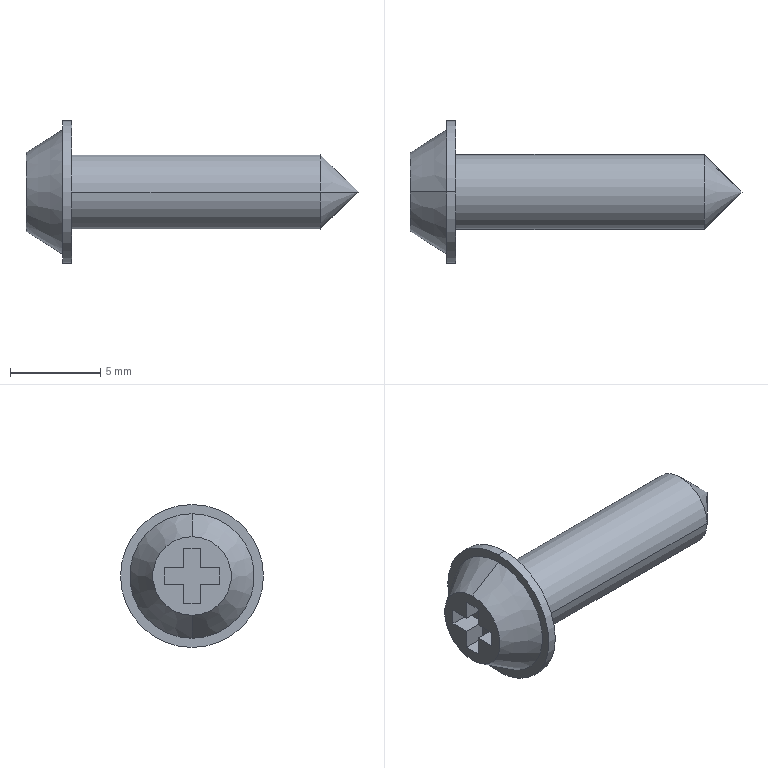Part | NX | features BREP 1 | 1 solid | 24 faces | box 18.415 x 7.925 x 7.925 mm | volume 268.123 mm3 | plane 16 | cylinder 4 | cone 4 | commonest cylinder face diameters 4.166 x2 7.925 x2
STEP:
#1=CARTESIAN_POINT('',(-15.875,2.083,0.));
#2=VERTEX_POINT('',#1);
#3=CARTESIAN_POINT('',(-2.083,2.083,0.));
#4=VERTEX_POINT('',#3);
#5=CARTESIAN_POINT('',(-2.083,2.083,0.));
#6=DIRECTION('',(-1.,0.,0.));
#7=VECTOR('',#6,1000.);
#8=LINE('',#5,#7);
#9=EDGE_CURVE('',#2,#4,#8,.F.);
#10=ORIENTED_EDGE('',*,*,#9,.T.);
#11=CARTESIAN_POINT('',(-2.083,-2.083,0.));
#12=VERTEX_POINT('',#11);
#13=CARTESIAN_POINT('',(-2.083,0.,0.));
#14=DIRECTION('',(-1.,0.,0.));
#15=DIRECTION('',(0.,1.,0.));
#16=AXIS2_PLACEMENT_3D('',#13,#14,#15);
#17=CIRCLE('',#16,2.083);
#18=EDGE_CURVE('',#4,#12,#17,.T.);
#19=ORIENTED_EDGE('',*,*,#18,.T.);
#20=CARTESIAN_POINT('',(-15.875,-2.083,0.));
#21=VERTEX_POINT('',#20);
#22=CARTESIAN_POINT('',(-2.083,-2.083,0.));
#23=DIRECTION('',(-1.,0.,0.));
#24=VECTOR('',#23,1000.);
#25=LINE('',#22,#24);
#26=EDGE_CURVE('',#21,#12,#25,.F.);
#27=ORIENTED_EDGE('',*,*,#26,.F.);
#28=CARTESIAN_POINT('',(-15.875,0.,0.));
#29=DIRECTION('',(-1.,0.,0.));
#30=DIRECTION('',(0.,1.,0.));
#31=AXIS2_PLACEMENT_3D('',#28,#29,#30);
#32=CIRCLE('',#31,2.083);
#33=EDGE_CURVE('',#2,#21,#32,.T.);
#34=ORIENTED_EDGE('',*,*,#33,.F.);
#35=EDGE_LOOP('',(#10,#19,#27,#34));
#36=FACE_BOUND('',#35,.T.);
#37=CARTESIAN_POINT('',(0.,0.,0.));
#38=DIRECTION('',(-1.,0.,0.));
#39=DIRECTION('',(0.,1.,0.));
#40=AXIS2_PLACEMENT_3D('',#37,#38,#39);
#41=CYLINDRICAL_SURFACE('',#40,2.083);
#42=ADVANCED_FACE('',(#36),#41,.T.);
#43=CARTESIAN_POINT('',(-15.875,0.,-3.962));
#44=VERTEX_POINT('',#43);
#45=CARTESIAN_POINT('',(-15.875,0.,3.962));
#46=VERTEX_POINT('',#45);
#47=CARTESIAN_POINT('',(-15.875,0.,0.));
#48=DIRECTION('',(-1.,0.,0.));
#49=DIRECTION('',(0.,0.,-1.));
#50=AXIS2_PLACEMENT_3D('',#47,#48,#49);
#51=CIRCLE('',#50,3.962);
#52=EDGE_CURVE('',#44,#46,#51,.T.);
#53=ORIENTED_EDGE('',*,*,#52,.F.);
#54=CARTESIAN_POINT('',(-15.875,0.,0.));
#55=DIRECTION('',(1.,0.,0.));
#56=DIRECTION('',(0.,0.,-1.));
#57=AXIS2_PLACEMENT_3D('',#54,#55,#56);
#58=CIRCLE('',#57,3.962);
#59=EDGE_CURVE('',#44,#46,#58,.T.);
#60=ORIENTED_EDGE('',*,*,#59,.T.);
#61=EDGE_LOOP('',(#53,#60));
#62=FACE_BOUND('',#61,.T.);
#63=CARTESIAN_POINT('',(-15.875,0.,0.));
#64=DIRECTION('',(-1.,0.,0.));
#65=DIRECTION('',(0.,-1.,0.));
#66=AXIS2_PLACEMENT_3D('',#63,#64,#65);
#67=CIRCLE('',#66,2.083);
#68=EDGE_CURVE('',#21,#2,#67,.T.);
#69=ORIENTED_EDGE('',*,*,#68,.T.);
#70=ORIENTED_EDGE('',*,*,#33,.T.);
#71=EDGE_LOOP('',(#69,#70));
#72=FACE_BOUND('',#71,.T.);
#73=CARTESIAN_POINT('',(-15.875,0.,0.));
#74=DIRECTION('',(-1.,0.,0.));
#75=DIRECTION('',(0.,0.,1.));
#76=AXIS2_PLACEMENT_3D('',#73,#74,#75);
#77=PLANE('',#76);
#78=ADVANCED_FACE('',(#62,#72),#77,.F.);
#79=CARTESIAN_POINT('',(-16.383,0.,-3.962));
#80=VERTEX_POINT('',#79);
#81=CARTESIAN_POINT('',(-16.383,0.,3.962));
#82=VERTEX_POINT('',#81);
#83=CARTESIAN_POINT('',(-16.383,0.,0.));
#84=DIRECTION('',(1.,0.,0.));
#85=DIRECTION('',(0.,0.,-1.));
#86=AXIS2_PLACEMENT_3D('',#83,#84,#85);
#87=CIRCLE('',#86,3.962);
#88=EDGE_CURVE('',#80,#82,#87,.T.);
#89=ORIENTED_EDGE('',*,*,#88,.T.);
#90=CARTESIAN_POINT('',(-16.383,0.,3.962));
#91=DIRECTION('',(1.,0.,0.));
#92=VECTOR('',#91,1000.);
#93=LINE('',#90,#92);
#94=EDGE_CURVE('',#82,#46,#93,.T.);
#95=ORIENTED_EDGE('',*,*,#94,.T.);
#96=ORIENTED_EDGE('',*,*,#59,.F.);
#97=CARTESIAN_POINT('',(-16.383,0.,-3.962));
#98=DIRECTION('',(1.,0.,0.));
#99=VECTOR('',#98,1000.);
#100=LINE('',#97,#99);
#101=EDGE_CURVE('',#80,#44,#100,.T.);
#102=ORIENTED_EDGE('',*,*,#101,.F.);
#103=EDGE_LOOP('',(#89,#95,#96,#102));
#104=FACE_BOUND('',#103,.T.);
#105=CARTESIAN_POINT('',(-15.748,0.,0.));
#106=DIRECTION('',(-1.,0.,0.));
#107=DIRECTION('',(0.,0.,1.));
#108=AXIS2_PLACEMENT_3D('',#105,#106,#107);
#109=CYLINDRICAL_SURFACE('',#108,3.962);
#110=ADVANCED_FACE('',(#104),#109,.T.);
#111=ORIENTED_EDGE('',*,*,#52,.T.);
#112=ORIENTED_EDGE('',*,*,#94,.F.);
#113=CARTESIAN_POINT('',(-16.383,0.,0.));
#114=DIRECTION('',(-1.,0.,0.));
#115=DIRECTION('',(0.,0.,-1.));
#116=AXIS2_PLACEMENT_3D('',#113,#114,#115);
#117=CIRCLE('',#116,3.962);
#118=EDGE_CURVE('',#80,#82,#117,.T.);
#119=ORIENTED_EDGE('',*,*,#118,.F.);
#120=ORIENTED_EDGE('',*,*,#101,.T.);
#121=EDGE_LOOP('',(#111,#112,#119,#120));
#122=FACE_BOUND('',#121,.T.);
#123=CARTESIAN_POINT('',(-15.748,0.,0.));
#124=DIRECTION('',(-1.,0.,0.));
#125=DIRECTION('',(0.,0.,1.));
#126=AXIS2_PLACEMENT_3D('',#123,#124,#125);
#127=CYLINDRICAL_SURFACE('',#126,3.962);
#128=ADVANCED_FACE('',(#122),#127,.T.);
#129=ORIENTED_EDGE('',*,*,#88,.F.);
#130=ORIENTED_EDGE('',*,*,#118,.T.);
#131=EDGE_LOOP('',(#129,#130));
#132=FACE_BOUND('',#131,.T.);
#133=CARTESIAN_POINT('',(-16.383,0.,-3.454));
#134=VERTEX_POINT('',#133);
#135=CARTESIAN_POINT('',(-16.383,0.,3.454));
#136=VERTEX_POINT('',#135);
#137=CARTESIAN_POINT('',(-16.383,0.,0.));
#138=DIRECTION('',(-1.,0.,0.));
#139=DIRECTION('',(0.,0.,-1.));
#140=AXIS2_PLACEMENT_3D('',#137,#138,#139);
#141=CIRCLE('',#140,3.454);
#142=EDGE_CURVE('',#134,#136,#141,.T.);
#143=ORIENTED_EDGE('',*,*,#142,.F.);
#144=CARTESIAN_POINT('',(-16.383,0.,0.));
#145=DIRECTION('',(1.,0.,0.));
#146=DIRECTION('',(0.,0.,-1.));
#147=AXIS2_PLACEMENT_3D('',#144,#145,#146);
#148=CIRCLE('',#147,3.454);
#149=EDGE_CURVE('',#134,#136,#148,.T.);
#150=ORIENTED_EDGE('',*,*,#149,.T.);
#151=EDGE_LOOP('',(#143,#150));
#152=FACE_BOUND('',#151,.T.);
#153=CARTESIAN_POINT('',(-16.383,0.,0.));
#154=DIRECTION('',(-1.,0.,0.));
#155=DIRECTION('',(0.,0.,1.));
#156=AXIS2_PLACEMENT_3D('',#153,#154,#155);
#157=PLANE('',#156);
#158=ADVANCED_FACE('',(#132,#152),#157,.T.);
#159=CARTESIAN_POINT('',(-18.415,0.,-2.179));
#160=VERTEX_POINT('',#159);
#161=CARTESIAN_POINT('',(-18.415,0.,2.179));
#162=VERTEX_POINT('',#161);
#163=CARTESIAN_POINT('',(-18.415,0.,0.));
#164=DIRECTION('',(1.,0.,0.));
#165=DIRECTION('',(0.,0.,-1.));
#166=AXIS2_PLACEMENT_3D('',#163,#164,#165);
#167=CIRCLE('',#166,2.179);
#168=EDGE_CURVE('',#160,#162,#167,.T.);
#169=ORIENTED_EDGE('',*,*,#168,.T.);
#170=CARTESIAN_POINT('',(-18.415,0.,2.179));
#171=DIRECTION('',(0.847,0.,0.5315));
#172=VECTOR('',#171,1000.);
#173=LINE('',#170,#172);
#174=EDGE_CURVE('',#162,#136,#173,.T.);
#175=ORIENTED_EDGE('',*,*,#174,.T.);
#176=ORIENTED_EDGE('',*,*,#149,.F.);
#177=CARTESIAN_POINT('',(-18.415,0.,-2.179));
#178=DIRECTION('',(0.847,0.,-0.5315));
#179=VECTOR('',#178,1000.);
#180=LINE('',#177,#179);
#181=EDGE_CURVE('',#160,#134,#180,.T.);
#182=ORIENTED_EDGE('',*,*,#181,.F.);
#183=EDGE_LOOP('',(#169,#175,#176,#182));
#184=FACE_BOUND('',#183,.T.);
#185=CARTESIAN_POINT('',(-17.399,0.,0.));
#186=DIRECTION('',(1.,0.,0.));
#187=DIRECTION('',(0.,0.,-1.));
#188=AXIS2_PLACEMENT_3D('',#185,#186,#187);
#189=CONICAL_SURFACE('',#188,2.817,0.5604);
#190=ADVANCED_FACE('',(#184),#189,.T.);
#191=ORIENTED_EDGE('',*,*,#142,.T.);
#192=ORIENTED_EDGE('',*,*,#174,.F.);
#193=CARTESIAN_POINT('',(-18.415,0.,0.));
#194=DIRECTION('',(-1.,0.,0.));
#195=DIRECTION('',(0.,0.,-1.));
#196=AXIS2_PLACEMENT_3D('',#193,#194,#195);
#197=CIRCLE('',#196,2.179);
#198=EDGE_CURVE('',#160,#162,#197,.T.);
#199=ORIENTED_EDGE('',*,*,#198,.F.);
#200=ORIENTED_EDGE('',*,*,#181,.T.);
#201=EDGE_LOOP('',(#191,#192,#199,#200));
#202=FACE_BOUND('',#201,.T.);
#203=CARTESIAN_POINT('',(-17.399,0.,0.));
#204=DIRECTION('',(1.,0.,0.));
#205=DIRECTION('',(0.,0.,-1.));
#206=AXIS2_PLACEMENT_3D('',#203,#204,#205);
#207=CONICAL_SURFACE('',#206,2.817,0.5604);
#208=ADVANCED_FACE('',(#202),#207,.T.);
#209=ORIENTED_EDGE('',*,*,#168,.F.);
#210=ORIENTED_EDGE('',*,*,#198,.T.);
#211=EDGE_LOOP('',(#209,#210));
#212=FACE_BOUND('',#211,.T.);
#213=CARTESIAN_POINT('',(-18.415,1.524,-0.4445));
#214=VERTEX_POINT('',#213);
#215=CARTESIAN_POINT('',(-18.415,1.524,0.4445));
#216=VERTEX_POINT('',#215);
#217=CARTESIAN_POINT('',(-18.415,1.524,-0.4445));
#218=DIRECTION('',(0.,0.,1.));
#219=VECTOR('',#218,1000.);
#220=LINE('',#217,#219);
#221=EDGE_CURVE('',#214,#216,#220,.T.);
#222=ORIENTED_EDGE('',*,*,#221,.T.);
#223=CARTESIAN_POINT('',(-18.415,0.4445,0.4445));
#224=VERTEX_POINT('',#223);
#225=CARTESIAN_POINT('',(-18.415,1.524,0.4445));
#226=DIRECTION('',(0.,-1.,0.));
#227=VECTOR('',#226,1000.);
#228=LINE('',#225,#227);
#229=EDGE_CURVE('',#216,#224,#228,.T.);
#230=ORIENTED_EDGE('',*,*,#229,.T.);
#231=CARTESIAN_POINT('',(-18.415,0.4445,1.524));
#232=VERTEX_POINT('',#231);
#233=CARTESIAN_POINT('',(-18.415,0.4445,0.4445));
#234=DIRECTION('',(0.,0.,1.));
#235=VECTOR('',#234,1000.);
#236=LINE('',#233,#235);
#237=EDGE_CURVE('',#224,#232,#236,.T.);
#238=ORIENTED_EDGE('',*,*,#237,.T.);
#239=CARTESIAN_POINT('',(-18.415,-0.4445,1.524));
#240=VERTEX_POINT('',#239);
#241=CARTESIAN_POINT('',(-18.415,0.4445,1.524));
#242=DIRECTION('',(0.,-1.,0.));
#243=VECTOR('',#242,1000.);
#244=LINE('',#241,#243);
#245=EDGE_CURVE('',#232,#240,#244,.T.);
#246=ORIENTED_EDGE('',*,*,#245,.T.);
#247=CARTESIAN_POINT('',(-18.415,-0.4445,0.4445));
#248=VERTEX_POINT('',#247);
#249=CARTESIAN_POINT('',(-18.415,-0.4445,1.524));
#250=DIRECTION('',(0.,0.,-1.));
#251=VECTOR('',#250,1000.);
#252=LINE('',#249,#251);
#253=EDGE_CURVE('',#240,#248,#252,.T.);
#254=ORIENTED_EDGE('',*,*,#253,.T.);
#255=CARTESIAN_POINT('',(-18.415,-1.524,0.4445));
#256=VERTEX_POINT('',#255);
#257=CARTESIAN_POINT('',(-18.415,-1.524,0.4445));
#258=DIRECTION('',(0.,1.,0.));
#259=VECTOR('',#258,1000.);
#260=LINE('',#257,#259);
#261=EDGE_CURVE('',#256,#248,#260,.T.);
#262=ORIENTED_EDGE('',*,*,#261,.F.);
#263=CARTESIAN_POINT('',(-18.415,-1.524,-0.4445));
#264=VERTEX_POINT('',#263);
#265=CARTESIAN_POINT('',(-18.415,-1.524,-0.4445));
#266=DIRECTION('',(0.,0.,1.));
#267=VECTOR('',#266,1000.);
#268=LINE('',#265,#267);
#269=EDGE_CURVE('',#264,#256,#268,.T.);
#270=ORIENTED_EDGE('',*,*,#269,.F.);
#271=CARTESIAN_POINT('',(-18.415,-0.4445,-0.4445));
#272=VERTEX_POINT('',#271);
#273=CARTESIAN_POINT('',(-18.415,-0.4445,-0.4445));
#274=DIRECTION('',(0.,-1.,0.));
#275=VECTOR('',#274,1000.);
#276=LINE('',#273,#275);
#277=EDGE_CURVE('',#272,#264,#276,.T.);
#278=ORIENTED_EDGE('',*,*,#277,.F.);
#279=CARTESIAN_POINT('',(-18.415,-0.4445,-1.524));
#280=VERTEX_POINT('',#279);
#281=CARTESIAN_POINT('',(-18.415,-0.4445,-0.4445));
#282=DIRECTION('',(0.,0.,-1.));
#283=VECTOR('',#282,1000.);
#284=LINE('',#281,#283);
#285=EDGE_CURVE('',#272,#280,#284,.T.);
#286=ORIENTED_EDGE('',*,*,#285,.T.);
#287=CARTESIAN_POINT('',(-18.415,0.4445,-1.524));
#288=VERTEX_POINT('',#287);
#289=CARTESIAN_POINT('',(-18.415,0.4445,-1.524));
#290=DIRECTION('',(0.,-1.,0.));
#291=VECTOR('',#290,1000.);
#292=LINE('',#289,#291);
#293=EDGE_CURVE('',#288,#280,#292,.T.);
#294=ORIENTED_EDGE('',*,*,#293,.F.);
#295=CARTESIAN_POINT('',(-18.415,0.4445,-0.4445));
#296=VERTEX_POINT('',#295);
#297=CARTESIAN_POINT('',(-18.415,0.4445,-1.524));
#298=DIRECTION('',(0.,0.,1.));
#299=VECTOR('',#298,1000.);
#300=LINE('',#297,#299);
#301=EDGE_CURVE('',#288,#296,#300,.T.);
#302=ORIENTED_EDGE('',*,*,#301,.T.);
#303=CARTESIAN_POINT('',(-18.415,0.4445,-0.4445));
#304=DIRECTION('',(0.,1.,0.));
#305=VECTOR('',#304,1000.);
#306=LINE('',#303,#305);
#307=EDGE_CURVE('',#296,#214,#306,.T.);
#308=ORIENTED_EDGE('',*,*,#307,.T.);
#309=EDGE_LOOP('',(#222,#230,#238,#246,#254,#262,#270,#278,#286,#294,#302,#308));
#310=FACE_BOUND('',#309,.T.);
#311=CARTESIAN_POINT('',(-18.415,0.,0.));
#312=DIRECTION('',(-1.,0.,0.));
#313=DIRECTION('',(0.,0.,1.));
#314=AXIS2_PLACEMENT_3D('',#311,#312,#313);
#315=PLANE('',#314);
#316=ADVANCED_FACE('',(#212,#310),#315,.T.);
#317=CARTESIAN_POINT('',(-17.145,0.4445,-0.4445));
#318=VERTEX_POINT('',#317);
#319=CARTESIAN_POINT('',(-17.145,0.4445,-0.4445));
#320=DIRECTION('',(-1.,0.,0.));
#321=VECTOR('',#320,1000.);
#322=LINE('',#319,#321);
#323=EDGE_CURVE('',#318,#296,#322,.T.);
#324=ORIENTED_EDGE('',*,*,#323,.F.);
#325=CARTESIAN_POINT('',(-17.145,1.524,-0.4445));
#326=VERTEX_POINT('',#325);
#327=CARTESIAN_POINT('',(-17.145,0.4445,-0.4445));
#328=DIRECTION('',(0.,1.,0.));
#329=VECTOR('',#328,1000.);
#330=LINE('',#327,#329);
#331=EDGE_CURVE('',#318,#326,#330,.T.);
#332=ORIENTED_EDGE('',*,*,#331,.T.);
#333=CARTESIAN_POINT('',(-18.415,1.524,-0.4445));
#334=DIRECTION('',(1.,0.,0.));
#335=VECTOR('',#334,1000.);
#336=LINE('',#333,#335);
#337=EDGE_CURVE('',#214,#326,#336,.T.);
#338=ORIENTED_EDGE('',*,*,#337,.F.);
#339=ORIENTED_EDGE('',*,*,#307,.F.);
#340=EDGE_LOOP('',(#324,#332,#338,#339));
#341=FACE_BOUND('',#340,.T.);
#342=CARTESIAN_POINT('',(-18.415,0.,-0.4445));
#343=DIRECTION('',(0.,0.,1.));
#344=DIRECTION('',(1.,0.,0.));
#345=AXIS2_PLACEMENT_3D('',#342,#343,#344);
#346=PLANE('',#345);
#347=ADVANCED_FACE('',(#341),#346,.T.);
#348=ORIENTED_EDGE('',*,*,#337,.T.);
#349=CARTESIAN_POINT('',(-17.145,1.524,0.4445));
#350=VERTEX_POINT('',#349);
#351=CARTESIAN_POINT('',(-17.145,1.524,-0.4445));
#352=DIRECTION('',(0.,0.,1.));
#353=VECTOR('',#352,1000.);
#354=LINE('',#351,#353);
#355=EDGE_CURVE('',#326,#350,#354,.T.);
#356=ORIENTED_EDGE('',*,*,#355,.T.);
#357=CARTESIAN_POINT('',(-18.415,1.524,0.4445));
#358=DIRECTION('',(1.,0.,0.));
#359=VECTOR('',#358,1000.);
#360=LINE('',#357,#359);
#361=EDGE_CURVE('',#216,#350,#360,.T.);
#362=ORIENTED_EDGE('',*,*,#361,.F.);
#363=ORIENTED_EDGE('',*,*,#221,.F.);
#364=EDGE_LOOP('',(#348,#356,#362,#363));
#365=FACE_BOUND('',#364,.T.);
#366=CARTESIAN_POINT('',(-18.415,1.524,-0.4445));
#367=DIRECTION('',(0.,-1.,0.));
#368=DIRECTION('',(0.,0.,-1.));
#369=AXIS2_PLACEMENT_3D('',#366,#367,#368);
#370=PLANE('',#369);
#371=ADVANCED_FACE('',(#365),#370,.T.);
#372=ORIENTED_EDGE('',*,*,#361,.T.);
#373=CARTESIAN_POINT('',(-17.145,0.4445,0.4445));
#374=VERTEX_POINT('',#373);
#375=CARTESIAN_POINT('',(-17.145,1.524,0.4445));
#376=DIRECTION('',(0.,-1.,0.));
#377=VECTOR('',#376,1000.);
#378=LINE('',#375,#377);
#379=EDGE_CURVE('',#350,#374,#378,.T.);
#380=ORIENTED_EDGE('',*,*,#379,.T.);
#381=CARTESIAN_POINT('',(-17.145,0.4445,0.4445));
#382=DIRECTION('',(-1.,0.,0.));
#383=VECTOR('',#382,1000.);
#384=LINE('',#381,#383);
#385=EDGE_CURVE('',#374,#224,#384,.T.);
#386=ORIENTED_EDGE('',*,*,#385,.T.);
#387=ORIENTED_EDGE('',*,*,#229,.F.);
#388=EDGE_LOOP('',(#372,#380,#386,#387));
#389=FACE_BOUND('',#388,.T.);
#390=CARTESIAN_POINT('',(-18.415,1.524,0.4445));
#391=DIRECTION('',(0.,0.,-1.));
#392=DIRECTION('',(0.,-1.,0.));
#393=AXIS2_PLACEMENT_3D('',#390,#391,#392);
#394=PLANE('',#393);
#395=ADVANCED_FACE('',(#389),#394,.T.);
#396=ORIENTED_EDGE('',*,*,#301,.F.);
#397=CARTESIAN_POINT('',(-17.145,0.4445,-1.524));
#398=VERTEX_POINT('',#397);
#399=CARTESIAN_POINT('',(-18.415,0.4445,-1.524));
#400=DIRECTION('',(1.,0.,0.));
#401=VECTOR('',#400,1000.);
#402=LINE('',#399,#401);
#403=EDGE_CURVE('',#288,#398,#402,.T.);
#404=ORIENTED_EDGE('',*,*,#403,.T.);
#405=CARTESIAN_POINT('',(-17.145,0.4445,-0.4445));
#406=DIRECTION('',(0.,0.,-1.));
#407=VECTOR('',#406,1000.);
#408=LINE('',#405,#407);
#409=EDGE_CURVE('',#318,#398,#408,.T.);
#410=ORIENTED_EDGE('',*,*,#409,.F.);
#411=ORIENTED_EDGE('',*,*,#323,.T.);
#412=EDGE_LOOP('',(#396,#404,#410,#411));
#413=FACE_BOUND('',#412,.T.);
#414=CARTESIAN_POINT('',(-18.415,0.4445,0.));
#415=DIRECTION('',(0.,1.,0.));
#416=DIRECTION('',(1.,0.,0.));
#417=AXIS2_PLACEMENT_3D('',#414,#415,#416);
#418=PLANE('',#417);
#419=ADVANCED_FACE('',(#413),#418,.F.);
#420=CARTESIAN_POINT('',(-17.145,0.4445,1.524));
#421=VERTEX_POINT('',#420);
#422=CARTESIAN_POINT('',(-17.145,0.4445,1.524));
#423=DIRECTION('',(0.,0.,-1.));
#424=VECTOR('',#423,1000.);
#425=LINE('',#422,#424);
#426=EDGE_CURVE('',#421,#374,#425,.T.);
#427=ORIENTED_EDGE('',*,*,#426,.F.);
#428=CARTESIAN_POINT('',(-18.415,0.4445,1.524));
#429=DIRECTION('',(1.,0.,0.));
#430=VECTOR('',#429,1000.);
#431=LINE('',#428,#430);
#432=EDGE_CURVE('',#232,#421,#431,.T.);
#433=ORIENTED_EDGE('',*,*,#432,.F.);
#434=ORIENTED_EDGE('',*,*,#237,.F.);
#435=ORIENTED_EDGE('',*,*,#385,.F.);
#436=EDGE_LOOP('',(#427,#433,#434,#435));
#437=FACE_BOUND('',#436,.T.);
#438=CARTESIAN_POINT('',(-18.415,0.4445,0.));
#439=DIRECTION('',(0.,1.,0.));
#440=DIRECTION('',(1.,0.,0.));
#441=AXIS2_PLACEMENT_3D('',#438,#439,#440);
#442=PLANE('',#441);
#443=ADVANCED_FACE('',(#437),#442,.F.);
#444=CARTESIAN_POINT('',(-17.145,-0.4445,-1.524));
#445=VERTEX_POINT('',#444);
#446=CARTESIAN_POINT('',(-17.145,0.4445,-1.524));
#447=DIRECTION('',(0.,-1.,0.));
#448=VECTOR('',#447,1000.);
#449=LINE('',#446,#448);
#450=EDGE_CURVE('',#398,#445,#449,.T.);
#451=ORIENTED_EDGE('',*,*,#450,.T.);
#452=CARTESIAN_POINT('',(-17.145,-0.4445,-0.4445));
#453=VERTEX_POINT('',#452);
#454=CARTESIAN_POINT('',(-17.145,-0.4445,-1.524));
#455=DIRECTION('',(0.,0.,1.));
#456=VECTOR('',#455,1000.);
#457=LINE('',#454,#456);
#458=EDGE_CURVE('',#445,#453,#457,.T.);
#459=ORIENTED_EDGE('',*,*,#458,.T.);
#460=CARTESIAN_POINT('',(-17.145,-1.524,-0.4445));
#461=VERTEX_POINT('',#460);
#462=CARTESIAN_POINT('',(-17.145,-0.4445,-0.4445));
#463=DIRECTION('',(0.,-1.,0.));
#464=VECTOR('',#463,1000.);
#465=LINE('',#462,#464);
#466=EDGE_CURVE('',#453,#461,#465,.T.);
#467=ORIENTED_EDGE('',*,*,#466,.T.);
#468=CARTESIAN_POINT('',(-17.145,-1.524,0.4445));
#469=VERTEX_POINT('',#468);
#470=CARTESIAN_POINT('',(-17.145,-1.524,-0.4445));
#471=DIRECTION('',(0.,0.,1.));
#472=VECTOR('',#471,1000.);
#473=LINE('',#470,#472);
#474=EDGE_CURVE('',#461,#469,#473,.T.);
#475=ORIENTED_EDGE('',*,*,#474,.T.);
#476=CARTESIAN_POINT('',(-17.145,-0.4445,0.4445));
#477=VERTEX_POINT('',#476);
#478=CARTESIAN_POINT('',(-17.145,-1.524,0.4445));
#479=DIRECTION('',(0.,1.,0.));
#480=VECTOR('',#479,1000.);
#481=LINE('',#478,#480);
#482=EDGE_CURVE('',#469,#477,#481,.T.);
#483=ORIENTED_EDGE('',*,*,#482,.T.);
#484=CARTESIAN_POINT('',(-17.145,-0.4445,1.524));
#485=VERTEX_POINT('',#484);
#486=CARTESIAN_POINT('',(-17.145,-0.4445,0.4445));
#487=DIRECTION('',(0.,0.,1.));
#488=VECTOR('',#487,1000.);
#489=LINE('',#486,#488);
#490=EDGE_CURVE('',#477,#485,#489,.T.);
#491=ORIENTED_EDGE('',*,*,#490,.T.);
#492=CARTESIAN_POINT('',(-17.145,0.4445,1.524));
#493=DIRECTION('',(0.,-1.,0.));
#494=VECTOR('',#493,1000.);
#495=LINE('',#492,#494);
#496=EDGE_CURVE('',#421,#485,#495,.T.);
#497=ORIENTED_EDGE('',*,*,#496,.F.);
#498=ORIENTED_EDGE('',*,*,#426,.T.);
#499=ORIENTED_EDGE('',*,*,#379,.F.);
#500=ORIENTED_EDGE('',*,*,#355,.F.);
#501=ORIENTED_EDGE('',*,*,#331,.F.);
#502=ORIENTED_EDGE('',*,*,#409,.T.);
#503=EDGE_LOOP('',(#451,#459,#467,#475,#483,#491,#497,#498,#499,#500,#501,#502));
#504=FACE_BOUND('',#503,.T.);
#505=CARTESIAN_POINT('',(-17.145,0.,0.));
#506=DIRECTION('',(-1.,0.,0.));
#507=DIRECTION('',(0.,0.,1.));
#508=AXIS2_PLACEMENT_3D('',#505,#506,#507);
#509=PLANE('',#508);
#510=ADVANCED_FACE('',(#504),#509,.T.);
#511=ORIENTED_EDGE('',*,*,#432,.T.);
#512=ORIENTED_EDGE('',*,*,#496,.T.);
#513=CARTESIAN_POINT('',(-18.415,-0.4445,1.524));
#514=DIRECTION('',(1.,0.,0.));
#515=VECTOR('',#514,1000.);
#516=LINE('',#513,#515);
#517=EDGE_CURVE('',#240,#485,#516,.T.);
#518=ORIENTED_EDGE('',*,*,#517,.F.);
#519=ORIENTED_EDGE('',*,*,#245,.F.);
#520=EDGE_LOOP('',(#511,#512,#518,#519));
#521=FACE_BOUND('',#520,.T.);
#522=CARTESIAN_POINT('',(-18.415,0.4445,1.524));
#523=DIRECTION('',(0.,0.,-1.));
#524=DIRECTION('',(0.,-1.,0.));
#525=AXIS2_PLACEMENT_3D('',#522,#523,#524);
#526=PLANE('',#525);
#527=ADVANCED_FACE('',(#521),#526,.T.);
#528=ORIENTED_EDGE('',*,*,#458,.F.);
#529=CARTESIAN_POINT('',(-18.415,-0.4445,-1.524));
#530=DIRECTION('',(1.,0.,0.));
#531=VECTOR('',#530,1000.);
#532=LINE('',#529,#531);
#533=EDGE_CURVE('',#280,#445,#532,.T.);
#534=ORIENTED_EDGE('',*,*,#533,.F.);
#535=ORIENTED_EDGE('',*,*,#285,.F.);
#536=CARTESIAN_POINT('',(-17.145,-0.4445,-0.4445));
#537=DIRECTION('',(-1.,0.,0.));
#538=VECTOR('',#537,1000.);
#539=LINE('',#536,#538);
#540=EDGE_CURVE('',#453,#272,#539,.T.);
#541=ORIENTED_EDGE('',*,*,#540,.F.);
#542=EDGE_LOOP('',(#528,#534,#535,#541));
#543=FACE_BOUND('',#542,.T.);
#544=CARTESIAN_POINT('',(-18.415,-0.4445,-1.524));
#545=DIRECTION('',(0.,-1.,0.));
#546=DIRECTION('',(0.,0.,-1.));
#547=AXIS2_PLACEMENT_3D('',#544,#545,#546);
#548=PLANE('',#547);
#549=ADVANCED_FACE('',(#543),#548,.F.);
#550=ORIENTED_EDGE('',*,*,#253,.F.);
#551=ORIENTED_EDGE('',*,*,#517,.T.);
#552=ORIENTED_EDGE('',*,*,#490,.F.);
#553=CARTESIAN_POINT('',(-17.145,-0.4445,0.4445));
#554=DIRECTION('',(-1.,0.,0.));
#555=VECTOR('',#554,1000.);
#556=LINE('',#553,#555);
#557=EDGE_CURVE('',#477,#248,#556,.T.);
#558=ORIENTED_EDGE('',*,*,#557,.T.);
#559=EDGE_LOOP('',(#550,#551,#552,#558));
#560=FACE_BOUND('',#559,.T.);
#561=CARTESIAN_POINT('',(-18.415,-0.4445,-1.524));
#562=DIRECTION('',(0.,-1.,0.));
#563=DIRECTION('',(0.,0.,-1.));
#564=AXIS2_PLACEMENT_3D('',#561,#562,#563);
#565=PLANE('',#564);
#566=ADVANCED_FACE('',(#560),#565,.F.);
#567=CARTESIAN_POINT('',(-18.415,-1.524,-0.4445));
#568=DIRECTION('',(1.,0.,0.));
#569=VECTOR('',#568,1000.);
#570=LINE('',#567,#569);
#571=EDGE_CURVE('',#264,#461,#570,.T.);
#572=ORIENTED_EDGE('',*,*,#571,.T.);
#573=ORIENTED_EDGE('',*,*,#466,.F.);
#574=ORIENTED_EDGE('',*,*,#540,.T.);
#575=ORIENTED_EDGE('',*,*,#277,.T.);
#576=EDGE_LOOP('',(#572,#573,#574,#575));
#577=FACE_BOUND('',#576,.T.);
#578=CARTESIAN_POINT('',(-18.415,0.,-0.4445));
#579=DIRECTION('',(0.,0.,-1.));
#580=DIRECTION('',(0.,-1.,0.));
#581=AXIS2_PLACEMENT_3D('',#578,#579,#580);
#582=PLANE('',#581);
#583=ADVANCED_FACE('',(#577),#582,.F.);
#584=CARTESIAN_POINT('',(-18.415,-1.524,0.4445));
#585=DIRECTION('',(1.,0.,0.));
#586=VECTOR('',#585,1000.);
#587=LINE('',#584,#586);
#588=EDGE_CURVE('',#256,#469,#587,.T.);
#589=ORIENTED_EDGE('',*,*,#588,.T.);
#590=ORIENTED_EDGE('',*,*,#474,.F.);
#591=ORIENTED_EDGE('',*,*,#571,.F.);
#592=ORIENTED_EDGE('',*,*,#269,.T.);
#593=EDGE_LOOP('',(#589,#590,#591,#592));
#594=FACE_BOUND('',#593,.T.);
#595=CARTESIAN_POINT('',(-18.415,-1.524,-0.4445));
#596=DIRECTION('',(0.,-1.,0.));
#597=DIRECTION('',(0.,0.,-1.));
#598=AXIS2_PLACEMENT_3D('',#595,#596,#597);
#599=PLANE('',#598);
#600=ADVANCED_FACE('',(#594),#599,.F.);
#601=ORIENTED_EDGE('',*,*,#557,.F.);
#602=ORIENTED_EDGE('',*,*,#482,.F.);
#603=ORIENTED_EDGE('',*,*,#588,.F.);
#604=ORIENTED_EDGE('',*,*,#261,.T.);
#605=EDGE_LOOP('',(#601,#602,#603,#604));
#606=FACE_BOUND('',#605,.T.);
#607=CARTESIAN_POINT('',(-18.415,-1.524,0.4445));
#608=DIRECTION('',(0.,0.,1.));
#609=DIRECTION('',(1.,0.,0.));
#610=AXIS2_PLACEMENT_3D('',#607,#608,#609);
#611=PLANE('',#610);
#612=ADVANCED_FACE('',(#606),#611,.F.);
#613=ORIENTED_EDGE('',*,*,#533,.T.);
#614=ORIENTED_EDGE('',*,*,#450,.F.);
#615=ORIENTED_EDGE('',*,*,#403,.F.);
#616=ORIENTED_EDGE('',*,*,#293,.T.);
#617=EDGE_LOOP('',(#613,#614,#615,#616));
#618=FACE_BOUND('',#617,.T.);
#619=CARTESIAN_POINT('',(-18.415,0.4445,-1.524));
#620=DIRECTION('',(0.,0.,-1.));
#621=DIRECTION('',(0.,-1.,0.));
#622=AXIS2_PLACEMENT_3D('',#619,#620,#621);
#623=PLANE('',#622);
#624=ADVANCED_FACE('',(#618),#623,.F.);
#625=ORIENTED_EDGE('',*,*,#26,.T.);
#626=CARTESIAN_POINT('',(-2.083,0.,0.));
#627=DIRECTION('',(-1.,0.,0.));
#628=DIRECTION('',(0.,-1.,0.));
#629=AXIS2_PLACEMENT_3D('',#626,#627,#628);
#630=CIRCLE('',#629,2.083);
#631=EDGE_CURVE('',#12,#4,#630,.T.);
#632=ORIENTED_EDGE('',*,*,#631,.T.);
#633=ORIENTED_EDGE('',*,*,#9,.F.);
#634=ORIENTED_EDGE('',*,*,#68,.F.);
#635=EDGE_LOOP('',(#625,#632,#633,#634));
#636=FACE_BOUND('',#635,.T.);
#637=CARTESIAN_POINT('',(0.,0.,0.));
#638=DIRECTION('',(-1.,0.,0.));
#639=DIRECTION('',(0.,1.,0.));
#640=AXIS2_PLACEMENT_3D('',#637,#638,#639);
#641=CYLINDRICAL_SURFACE('',#640,2.083);
#642=ADVANCED_FACE('',(#636),#641,.T.);
#643=ORIENTED_EDGE('',*,*,#631,.F.);
#644=CARTESIAN_POINT('',(0.,0.,0.));
#645=VERTEX_POINT('',#644);
#646=CARTESIAN_POINT('',(0.,0.,0.));
#647=DIRECTION('',(-0.7071,-0.7071,0.));
#648=VECTOR('',#647,1000.);
#649=LINE('',#646,#648);
#650=EDGE_CURVE('',#645,#12,#649,.T.);
#651=ORIENTED_EDGE('',*,*,#650,.F.);
#652=CARTESIAN_POINT('',(0.,0.,0.));
#653=DIRECTION('',(-0.7071,0.7071,0.));
#654=VECTOR('',#653,1000.);
#655=LINE('',#652,#654);
#656=EDGE_CURVE('',#645,#4,#655,.T.);
#657=ORIENTED_EDGE('',*,*,#656,.T.);
#658=EDGE_LOOP('',(#643,#651,#657));
#659=FACE_BOUND('',#658,.T.);
#660=CARTESIAN_POINT('',(-1.062,0.,0.));
#661=DIRECTION('',(-1.,0.,0.));
#662=DIRECTION('',(0.,1.,0.));
#663=AXIS2_PLACEMENT_3D('',#660,#661,#662);
#664=CONICAL_SURFACE('',#663,1.062,0.7854);
#665=ADVANCED_FACE('',(#659),#664,.T.);
#666=ORIENTED_EDGE('',*,*,#18,.F.);
#667=ORIENTED_EDGE('',*,*,#656,.F.);
#668=ORIENTED_EDGE('',*,*,#650,.T.);
#669=EDGE_LOOP('',(#666,#667,#668));
#670=FACE_BOUND('',#669,.T.);
#671=CARTESIAN_POINT('',(-1.062,0.,0.));
#672=DIRECTION('',(-1.,0.,0.));
#673=DIRECTION('',(0.,1.,0.));
#674=AXIS2_PLACEMENT_3D('',#671,#672,#673);
#675=CONICAL_SURFACE('',#674,1.062,0.7854);
#676=ADVANCED_FACE('',(#670),#675,.T.);
#677=CLOSED_SHELL('',(#42,#78,#110,#128,#158,#190,#208,#316,#347,#371,#395,#419,#443,#510,#527,#549,#566,#583,#600,#612,#624,#642,#665,#676));
#678=MANIFOLD_SOLID_BREP('',#677);
#679=(LENGTH_UNIT()NAMED_UNIT(*)SI_UNIT(.MILLI.,.METRE.));
#680=UNCERTAINTY_MEASURE_WITH_UNIT(LENGTH_MEASURE(0.00001),#679,'','');
#681=(NAMED_UNIT(*)PLANE_ANGLE_UNIT()SI_UNIT($,.RADIAN.));
#682=(NAMED_UNIT(*)SI_UNIT($,.STERADIAN.)SOLID_ANGLE_UNIT());
#683=(GEOMETRIC_REPRESENTATION_CONTEXT(3)GLOBAL_UNCERTAINTY_ASSIGNED_CONTEXT((#680))GLOBAL_UNIT_ASSIGNED_CONTEXT((#679,#681,#682))REPRESENTATION_CONTEXT('',''));
#684=ADVANCED_BREP_SHAPE_REPRESENTATION('',(#678),#683);